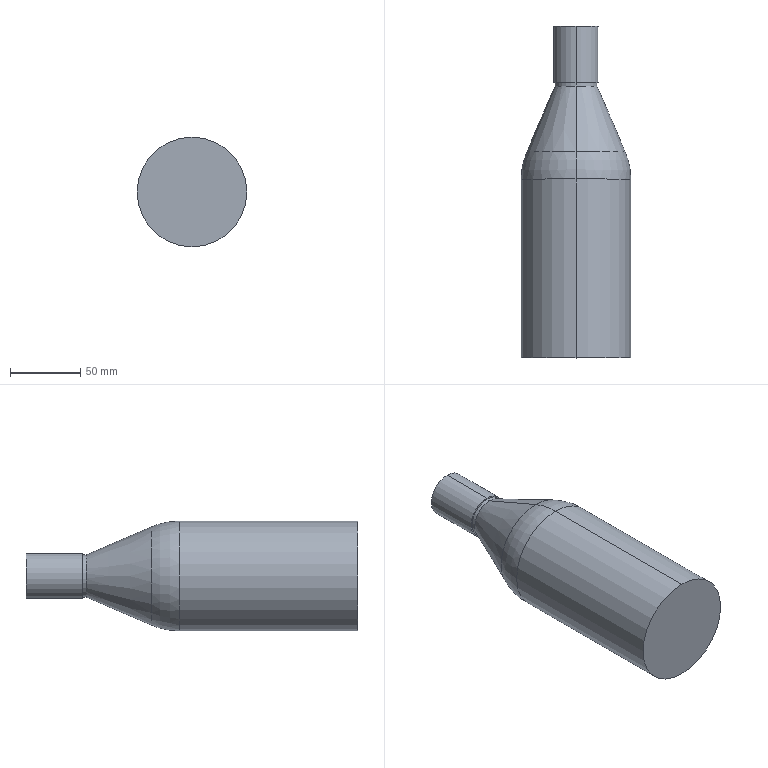Part | SolidWorks | features ICE 2, Revolution 1 | 1 solid | 21 faces | box 78 x 236 x 78 mm | volume 361829 mm3 | cylinder 10 | plane 5 | cone 4 | torus 2 | commonest cylinder face diameters 14 x2 30 x2 32 x2 62 x2 78 x2
STEP:
#1=CARTESIAN_POINT('',(0.,236.,16.));
#2=VERTEX_POINT('',#1);
#3=CARTESIAN_POINT('',(0.,236.,-16.));
#4=VERTEX_POINT('',#3);
#5=CARTESIAN_POINT('',(0.,236.,0.));
#6=DIRECTION('',(0.,1.,0.));
#7=DIRECTION('',(0.,0.,1.));
#8=AXIS2_PLACEMENT_3D('',#5,#6,#7);
#9=CIRCLE('',#8,16.);
#10=EDGE_CURVE('',#2,#4,#9,.T.);
#11=ORIENTED_EDGE('',*,*,#10,.F.);
#12=CARTESIAN_POINT('',(0.,196.,16.));
#13=VERTEX_POINT('',#12);
#14=CARTESIAN_POINT('',(0.,281.255,16.));
#15=DIRECTION('',(0.,-1.,0.));
#16=VECTOR('',#15,1000.);
#17=LINE('',#14,#16);
#18=EDGE_CURVE('',#2,#13,#17,.T.);
#19=ORIENTED_EDGE('',*,*,#18,.T.);
#20=CARTESIAN_POINT('',(0.,196.,-16.));
#21=VERTEX_POINT('',#20);
#22=CARTESIAN_POINT('',(0.,196.,0.));
#23=DIRECTION('',(0.,1.,0.));
#24=DIRECTION('',(0.,0.,1.));
#25=AXIS2_PLACEMENT_3D('',#22,#23,#24);
#26=CIRCLE('',#25,16.);
#27=EDGE_CURVE('',#13,#21,#26,.T.);
#28=ORIENTED_EDGE('',*,*,#27,.T.);
#29=CARTESIAN_POINT('',(0.,281.255,-16.));
#30=DIRECTION('',(0.,-1.,0.));
#31=VECTOR('',#30,1000.);
#32=LINE('',#29,#31);
#33=EDGE_CURVE('',#4,#21,#32,.T.);
#34=ORIENTED_EDGE('',*,*,#33,.F.);
#35=EDGE_LOOP('',(#11,#19,#28,#34));
#36=FACE_OUTER_BOUND('',#35,.T.);
#37=CARTESIAN_POINT('',(0.,281.255,0.));
#38=DIRECTION('',(0.,-1.,0.));
#39=DIRECTION('',(0.,0.,-1.));
#40=AXIS2_PLACEMENT_3D('',#37,#38,#39);
#41=CYLINDRICAL_SURFACE('',#40,16.);
#42=ADVANCED_FACE('',(#36),#41,.T.);
#43=CARTESIAN_POINT('',(0.,193.291,-15.));
#44=VERTEX_POINT('',#43);
#45=CARTESIAN_POINT('',(0.,193.291,15.));
#46=VERTEX_POINT('',#45);
#47=CARTESIAN_POINT('',(0.,193.291,0.));
#48=DIRECTION('',(0.,-1.,0.));
#49=DIRECTION('',(0.,0.,-1.));
#50=AXIS2_PLACEMENT_3D('',#47,#48,#49);
#51=CIRCLE('',#50,15.);
#52=EDGE_CURVE('',#44,#46,#51,.T.);
#53=ORIENTED_EDGE('',*,*,#52,.T.);
#54=CARTESIAN_POINT('',(0.,146.915,34.936));
#55=VERTEX_POINT('',#54);
#56=CARTESIAN_POINT('',(0.,146.915,34.936));
#57=DIRECTION('',(0.,-0.9187,0.3949));
#58=VECTOR('',#57,1000.);
#59=LINE('',#56,#58);
#60=EDGE_CURVE('',#46,#55,#59,.T.);
#61=ORIENTED_EDGE('',*,*,#60,.T.);
#62=CARTESIAN_POINT('',(0.,146.915,-34.936));
#63=VERTEX_POINT('',#62);
#64=CARTESIAN_POINT('',(0.,146.915,0.));
#65=DIRECTION('',(0.,-1.,0.));
#66=DIRECTION('',(0.,0.,-1.));
#67=AXIS2_PLACEMENT_3D('',#64,#65,#66);
#68=CIRCLE('',#67,34.936);
#69=EDGE_CURVE('',#63,#55,#68,.T.);
#70=ORIENTED_EDGE('',*,*,#69,.F.);
#71=CARTESIAN_POINT('',(0.,146.915,-34.936));
#72=DIRECTION('',(0.,-0.9187,-0.3949));
#73=VECTOR('',#72,1000.);
#74=LINE('',#71,#73);
#75=EDGE_CURVE('',#44,#63,#74,.T.);
#76=ORIENTED_EDGE('',*,*,#75,.F.);
#77=EDGE_LOOP('',(#53,#61,#70,#76));
#78=FACE_OUTER_BOUND('',#77,.T.);
#79=CARTESIAN_POINT('',(0.,146.915,0.));
#80=DIRECTION('',(0.,-1.,0.));
#81=DIRECTION('',(0.,0.,-1.));
#82=AXIS2_PLACEMENT_3D('',#79,#80,#81);
#83=CONICAL_SURFACE('',#82,34.936,0.406);
#84=ADVANCED_FACE('',(#78),#83,.T.);
#85=ORIENTED_EDGE('',*,*,#69,.T.);
#86=CARTESIAN_POINT('',(0.,127.169,39.));
#87=VERTEX_POINT('',#86);
#88=CARTESIAN_POINT('',(0.,127.169,-11.));
#89=DIRECTION('',(1.,0.,0.));
#90=DIRECTION('',(0.,0.,-1.));
#91=AXIS2_PLACEMENT_3D('',#88,#89,#90);
#92=CIRCLE('',#91,50.);
#93=EDGE_CURVE('',#55,#87,#92,.T.);
#94=ORIENTED_EDGE('',*,*,#93,.T.);
#95=CARTESIAN_POINT('',(0.,127.169,-39.));
#96=VERTEX_POINT('',#95);
#97=CARTESIAN_POINT('',(0.,127.169,0.));
#98=DIRECTION('',(0.,-1.,0.));
#99=DIRECTION('',(0.,0.,-1.));
#100=AXIS2_PLACEMENT_3D('',#97,#98,#99);
#101=CIRCLE('',#100,39.);
#102=EDGE_CURVE('',#96,#87,#101,.T.);
#103=ORIENTED_EDGE('',*,*,#102,.F.);
#104=CARTESIAN_POINT('',(0.,127.169,11.));
#105=DIRECTION('',(-1.,0.,0.));
#106=DIRECTION('',(0.,0.,1.));
#107=AXIS2_PLACEMENT_3D('',#104,#105,#106);
#108=CIRCLE('',#107,50.);
#109=EDGE_CURVE('',#63,#96,#108,.T.);
#110=ORIENTED_EDGE('',*,*,#109,.F.);
#111=EDGE_LOOP('',(#85,#94,#103,#110));
#112=FACE_OUTER_BOUND('',#111,.T.);
#113=CARTESIAN_POINT('',(0.,127.169,0.));
#114=DIRECTION('',(0.,-1.,0.));
#115=DIRECTION('',(0.,0.,-1.));
#116=AXIS2_PLACEMENT_3D('',#113,#114,#115);
#117=TOROIDAL_SURFACE('',#116,-11.,50.);
#118=ADVANCED_FACE('',(#112),#117,.T.);
#119=ORIENTED_EDGE('',*,*,#102,.T.);
#120=CARTESIAN_POINT('',(0.,0.,39.));
#121=VERTEX_POINT('',#120);
#122=CARTESIAN_POINT('',(0.,0.,39.));
#123=DIRECTION('',(0.,-1.,0.));
#124=VECTOR('',#123,1000.);
#125=LINE('',#122,#124);
#126=EDGE_CURVE('',#87,#121,#125,.T.);
#127=ORIENTED_EDGE('',*,*,#126,.T.);
#128=CARTESIAN_POINT('',(0.,0.,-39.));
#129=VERTEX_POINT('',#128);
#130=CARTESIAN_POINT('',(0.,0.,0.));
#131=DIRECTION('',(0.,-1.,0.));
#132=DIRECTION('',(0.,0.,-1.));
#133=AXIS2_PLACEMENT_3D('',#130,#131,#132);
#134=CIRCLE('',#133,39.);
#135=EDGE_CURVE('',#129,#121,#134,.T.);
#136=ORIENTED_EDGE('',*,*,#135,.F.);
#137=CARTESIAN_POINT('',(0.,0.,-39.));
#138=DIRECTION('',(0.,-1.,0.));
#139=VECTOR('',#138,1000.);
#140=LINE('',#137,#139);
#141=EDGE_CURVE('',#96,#129,#140,.T.);
#142=ORIENTED_EDGE('',*,*,#141,.F.);
#143=EDGE_LOOP('',(#119,#127,#136,#142));
#144=FACE_OUTER_BOUND('',#143,.T.);
#145=CARTESIAN_POINT('',(0.,0.,0.));
#146=DIRECTION('',(0.,-1.,0.));
#147=DIRECTION('',(0.,0.,-1.));
#148=AXIS2_PLACEMENT_3D('',#145,#146,#147);
#149=CYLINDRICAL_SURFACE('',#148,39.);
#150=ADVANCED_FACE('',(#144),#149,.T.);
#151=CARTESIAN_POINT('',(0.,196.,15.));
#152=VERTEX_POINT('',#151);
#153=CARTESIAN_POINT('',(0.,196.,-15.));
#154=VERTEX_POINT('',#153);
#155=CARTESIAN_POINT('',(0.,196.,0.));
#156=DIRECTION('',(0.,1.,0.));
#157=DIRECTION('',(0.,0.,1.));
#158=AXIS2_PLACEMENT_3D('',#155,#156,#157);
#159=CIRCLE('',#158,15.);
#160=EDGE_CURVE('',#152,#154,#159,.T.);
#161=ORIENTED_EDGE('',*,*,#160,.F.);
#162=CARTESIAN_POINT('',(0.,0.,15.));
#163=DIRECTION('',(0.,-1.,0.));
#164=VECTOR('',#163,1000.);
#165=LINE('',#162,#164);
#166=EDGE_CURVE('',#152,#46,#165,.T.);
#167=ORIENTED_EDGE('',*,*,#166,.T.);
#168=ORIENTED_EDGE('',*,*,#52,.F.);
#169=CARTESIAN_POINT('',(0.,0.,-15.));
#170=DIRECTION('',(0.,-1.,0.));
#171=VECTOR('',#170,1000.);
#172=LINE('',#169,#171);
#173=EDGE_CURVE('',#154,#44,#172,.T.);
#174=ORIENTED_EDGE('',*,*,#173,.F.);
#175=EDGE_LOOP('',(#161,#167,#168,#174));
#176=FACE_OUTER_BOUND('',#175,.T.);
#177=CARTESIAN_POINT('',(0.,0.,0.));
#178=DIRECTION('',(0.,-1.,0.));
#179=DIRECTION('',(0.,0.,-1.));
#180=AXIS2_PLACEMENT_3D('',#177,#178,#179);
#181=CYLINDRICAL_SURFACE('',#180,15.);
#182=ADVANCED_FACE('',(#176),#181,.T.);
#183=ORIENTED_EDGE('',*,*,#166,.F.);
#184=CARTESIAN_POINT('',(0.,196.,0.));
#185=DIRECTION('',(0.,1.,0.));
#186=DIRECTION('',(0.,0.,1.));
#187=AXIS2_PLACEMENT_3D('',#184,#185,#186);
#188=CIRCLE('',#187,15.);
#189=EDGE_CURVE('',#154,#152,#188,.T.);
#190=ORIENTED_EDGE('',*,*,#189,.F.);
#191=ORIENTED_EDGE('',*,*,#173,.T.);
#192=CARTESIAN_POINT('',(0.,193.291,0.));
#193=DIRECTION('',(0.,-1.,0.));
#194=DIRECTION('',(0.,0.,-1.));
#195=AXIS2_PLACEMENT_3D('',#192,#193,#194);
#196=CIRCLE('',#195,15.);
#197=EDGE_CURVE('',#46,#44,#196,.T.);
#198=ORIENTED_EDGE('',*,*,#197,.F.);
#199=EDGE_LOOP('',(#183,#190,#191,#198));
#200=FACE_OUTER_BOUND('',#199,.T.);
#201=CARTESIAN_POINT('',(0.,0.,0.));
#202=DIRECTION('',(0.,-1.,0.));
#203=DIRECTION('',(0.,0.,-1.));
#204=AXIS2_PLACEMENT_3D('',#201,#202,#203);
#205=CYLINDRICAL_SURFACE('',#204,15.);
#206=ADVANCED_FACE('',(#200),#205,.T.);
#207=ORIENTED_EDGE('',*,*,#135,.T.);
#208=CARTESIAN_POINT('',(0.,0.,0.));
#209=DIRECTION('',(0.,-1.,0.));
#210=DIRECTION('',(0.,0.,-1.));
#211=AXIS2_PLACEMENT_3D('',#208,#209,#210);
#212=CIRCLE('',#211,39.);
#213=EDGE_CURVE('',#121,#129,#212,.T.);
#214=ORIENTED_EDGE('',*,*,#213,.T.);
#215=EDGE_LOOP('',(#207,#214));
#216=FACE_OUTER_BOUND('',#215,.T.);
#217=CARTESIAN_POINT('',(0.,0.,0.));
#218=DIRECTION('',(0.,-1.,0.));
#219=DIRECTION('',(0.,0.,-1.));
#220=AXIS2_PLACEMENT_3D('',#217,#218,#219);
#221=PLANE('',#220);
#222=ADVANCED_FACE('',(#216),#221,.T.);
#223=ORIENTED_EDGE('',*,*,#126,.F.);
#224=CARTESIAN_POINT('',(0.,127.169,0.));
#225=DIRECTION('',(0.,-1.,0.));
#226=DIRECTION('',(0.,0.,-1.));
#227=AXIS2_PLACEMENT_3D('',#224,#225,#226);
#228=CIRCLE('',#227,39.);
#229=EDGE_CURVE('',#87,#96,#228,.T.);
#230=ORIENTED_EDGE('',*,*,#229,.T.);
#231=ORIENTED_EDGE('',*,*,#141,.T.);
#232=ORIENTED_EDGE('',*,*,#213,.F.);
#233=EDGE_LOOP('',(#223,#230,#231,#232));
#234=FACE_OUTER_BOUND('',#233,.T.);
#235=CARTESIAN_POINT('',(0.,0.,0.));
#236=DIRECTION('',(0.,-1.,0.));
#237=DIRECTION('',(0.,0.,-1.));
#238=AXIS2_PLACEMENT_3D('',#235,#236,#237);
#239=CYLINDRICAL_SURFACE('',#238,39.);
#240=ADVANCED_FACE('',(#234),#239,.T.);
#241=ORIENTED_EDGE('',*,*,#93,.F.);
#242=CARTESIAN_POINT('',(0.,146.915,0.));
#243=DIRECTION('',(0.,-1.,0.));
#244=DIRECTION('',(0.,0.,-1.));
#245=AXIS2_PLACEMENT_3D('',#242,#243,#244);
#246=CIRCLE('',#245,34.936);
#247=EDGE_CURVE('',#55,#63,#246,.T.);
#248=ORIENTED_EDGE('',*,*,#247,.T.);
#249=ORIENTED_EDGE('',*,*,#109,.T.);
#250=ORIENTED_EDGE('',*,*,#229,.F.);
#251=EDGE_LOOP('',(#241,#248,#249,#250));
#252=FACE_OUTER_BOUND('',#251,.T.);
#253=CARTESIAN_POINT('',(0.,127.169,0.));
#254=DIRECTION('',(0.,-1.,0.));
#255=DIRECTION('',(0.,0.,-1.));
#256=AXIS2_PLACEMENT_3D('',#253,#254,#255);
#257=TOROIDAL_SURFACE('',#256,-11.,50.);
#258=ADVANCED_FACE('',(#252),#257,.T.);
#259=ORIENTED_EDGE('',*,*,#60,.F.);
#260=ORIENTED_EDGE('',*,*,#197,.T.);
#261=ORIENTED_EDGE('',*,*,#75,.T.);
#262=ORIENTED_EDGE('',*,*,#247,.F.);
#263=EDGE_LOOP('',(#259,#260,#261,#262));
#264=FACE_OUTER_BOUND('',#263,.T.);
#265=CARTESIAN_POINT('',(0.,146.915,0.));
#266=DIRECTION('',(0.,-1.,0.));
#267=DIRECTION('',(0.,0.,-1.));
#268=AXIS2_PLACEMENT_3D('',#265,#266,#267);
#269=CONICAL_SURFACE('',#268,34.936,0.406);
#270=ADVANCED_FACE('',(#264),#269,.T.);
#271=ORIENTED_EDGE('',*,*,#18,.F.);
#272=CARTESIAN_POINT('',(0.,236.,0.));
#273=DIRECTION('',(0.,1.,0.));
#274=DIRECTION('',(0.,0.,1.));
#275=AXIS2_PLACEMENT_3D('',#272,#273,#274);
#276=CIRCLE('',#275,16.);
#277=EDGE_CURVE('',#4,#2,#276,.T.);
#278=ORIENTED_EDGE('',*,*,#277,.F.);
#279=ORIENTED_EDGE('',*,*,#33,.T.);
#280=CARTESIAN_POINT('',(0.,196.,0.));
#281=DIRECTION('',(0.,1.,0.));
#282=DIRECTION('',(0.,0.,1.));
#283=AXIS2_PLACEMENT_3D('',#280,#281,#282);
#284=CIRCLE('',#283,16.);
#285=EDGE_CURVE('',#21,#13,#284,.T.);
#286=ORIENTED_EDGE('',*,*,#285,.T.);
#287=EDGE_LOOP('',(#271,#278,#279,#286));
#288=FACE_OUTER_BOUND('',#287,.T.);
#289=CARTESIAN_POINT('',(0.,281.255,0.));
#290=DIRECTION('',(0.,-1.,0.));
#291=DIRECTION('',(0.,0.,-1.));
#292=AXIS2_PLACEMENT_3D('',#289,#290,#291);
#293=CYLINDRICAL_SURFACE('',#292,16.);
#294=ADVANCED_FACE('',(#288),#293,.T.);
#295=ORIENTED_EDGE('',*,*,#285,.F.);
#296=ORIENTED_EDGE('',*,*,#27,.F.);
#297=EDGE_LOOP('',(#295,#296));
#298=FACE_OUTER_BOUND('',#297,.T.);
#299=ORIENTED_EDGE('',*,*,#189,.T.);
#300=ORIENTED_EDGE('',*,*,#160,.T.);
#301=EDGE_LOOP('',(#299,#300));
#302=FACE_BOUND('',#301,.T.);
#303=CARTESIAN_POINT('',(0.,196.,0.));
#304=DIRECTION('',(0.,1.,0.));
#305=DIRECTION('',(0.,0.,1.));
#306=AXIS2_PLACEMENT_3D('',#303,#304,#305);
#307=PLANE('',#306);
#308=ADVANCED_FACE('',(#298,#302),#307,.F.);
#309=ORIENTED_EDGE('',*,*,#277,.T.);
#310=ORIENTED_EDGE('',*,*,#10,.T.);
#311=EDGE_LOOP('',(#309,#310));
#312=FACE_OUTER_BOUND('',#311,.T.);
#313=CARTESIAN_POINT('',(7.,236.,0.));
#314=DIRECTION('',(0.,1.,0.));
#315=DIRECTION('',(0.,0.,1.));
#316=AXIS2_PLACEMENT_3D('',#313,#314,#315);
#317=PLANE('',#316);
#318=ADVANCED_FACE('',(#312),#317,.T.);
#319=CLOSED_SHELL('',(#42,#84,#118,#150,#182,#206,#222,#240,#258,#270,#294,#308,#318));
#320=CARTESIAN_POINT('',(0.,231.,-7.));
#321=VERTEX_POINT('',#320);
#322=CARTESIAN_POINT('',(0.,231.,7.));
#323=VERTEX_POINT('',#322);
#324=CARTESIAN_POINT('',(0.,231.,0.));
#325=DIRECTION('',(0.,1.,0.));
#326=DIRECTION('',(0.,0.,1.));
#327=AXIS2_PLACEMENT_3D('',#324,#325,#326);
#328=CIRCLE('',#327,7.);
#329=EDGE_CURVE('',#321,#323,#328,.T.);
#330=ORIENTED_EDGE('',*,*,#329,.T.);
#331=CARTESIAN_POINT('',(0.,191.644,7.));
#332=VERTEX_POINT('',#331);
#333=CARTESIAN_POINT('',(0.,0.,7.));
#334=DIRECTION('',(0.,-1.,0.));
#335=VECTOR('',#334,1000.);
#336=LINE('',#333,#335);
#337=EDGE_CURVE('',#323,#332,#336,.T.);
#338=ORIENTED_EDGE('',*,*,#337,.T.);
#339=CARTESIAN_POINT('',(0.,191.644,-7.));
#340=VERTEX_POINT('',#339);
#341=CARTESIAN_POINT('',(0.,191.644,0.));
#342=DIRECTION('',(0.,-1.,0.));
#343=DIRECTION('',(0.,0.,-1.));
#344=AXIS2_PLACEMENT_3D('',#341,#342,#343);
#345=CIRCLE('',#344,7.);
#346=EDGE_CURVE('',#332,#340,#345,.T.);
#347=ORIENTED_EDGE('',*,*,#346,.T.);
#348=CARTESIAN_POINT('',(0.,0.,-7.));
#349=DIRECTION('',(0.,-1.,0.));
#350=VECTOR('',#349,1000.);
#351=LINE('',#348,#350);
#352=EDGE_CURVE('',#321,#340,#351,.T.);
#353=ORIENTED_EDGE('',*,*,#352,.F.);
#354=EDGE_LOOP('',(#330,#338,#347,#353));
#355=FACE_OUTER_BOUND('',#354,.T.);
#356=CARTESIAN_POINT('',(0.,0.,0.));
#357=DIRECTION('',(0.,-1.,0.));
#358=DIRECTION('',(0.,0.,-1.));
#359=AXIS2_PLACEMENT_3D('',#356,#357,#358);
#360=CYLINDRICAL_SURFACE('',#359,7.);
#361=ADVANCED_FACE('',(#355),#360,.F.);
#362=ORIENTED_EDGE('',*,*,#346,.F.);
#363=CARTESIAN_POINT('',(0.,135.813,31.));
#364=VERTEX_POINT('',#363);
#365=CARTESIAN_POINT('',(0.,191.644,7.));
#366=DIRECTION('',(0.,-0.9187,0.3949));
#367=VECTOR('',#366,1000.);
#368=LINE('',#365,#367);
#369=EDGE_CURVE('',#332,#364,#368,.T.);
#370=ORIENTED_EDGE('',*,*,#369,.T.);
#371=CARTESIAN_POINT('',(0.,135.813,-31.));
#372=VERTEX_POINT('',#371);
#373=CARTESIAN_POINT('',(0.,135.813,0.));
#374=DIRECTION('',(0.,-1.,0.));
#375=DIRECTION('',(0.,0.,-1.));
#376=AXIS2_PLACEMENT_3D('',#373,#374,#375);
#377=CIRCLE('',#376,31.);
#378=EDGE_CURVE('',#364,#372,#377,.T.);
#379=ORIENTED_EDGE('',*,*,#378,.T.);
#380=CARTESIAN_POINT('',(0.,191.644,-7.));
#381=DIRECTION('',(0.,-0.9187,-0.3949));
#382=VECTOR('',#381,1000.);
#383=LINE('',#380,#382);
#384=EDGE_CURVE('',#340,#372,#383,.T.);
#385=ORIENTED_EDGE('',*,*,#384,.F.);
#386=EDGE_LOOP('',(#362,#370,#379,#385));
#387=FACE_OUTER_BOUND('',#386,.T.);
#388=CARTESIAN_POINT('',(0.,191.644,0.));
#389=DIRECTION('',(0.,-1.,0.));
#390=DIRECTION('',(0.,0.,-1.));
#391=AXIS2_PLACEMENT_3D('',#388,#389,#390);
#392=CONICAL_SURFACE('',#391,7.,0.406);
#393=ADVANCED_FACE('',(#387),#392,.F.);
#394=ORIENTED_EDGE('',*,*,#378,.F.);
#395=CARTESIAN_POINT('',(0.,8.,31.));
#396=VERTEX_POINT('',#395);
#397=CARTESIAN_POINT('',(0.,0.,31.));
#398=DIRECTION('',(0.,-1.,0.));
#399=VECTOR('',#398,1000.);
#400=LINE('',#397,#399);
#401=EDGE_CURVE('',#364,#396,#400,.T.);
#402=ORIENTED_EDGE('',*,*,#401,.T.);
#403=CARTESIAN_POINT('',(0.,8.,-31.));
#404=VERTEX_POINT('',#403);
#405=CARTESIAN_POINT('',(0.,8.,0.));
#406=DIRECTION('',(0.,-1.,0.));
#407=DIRECTION('',(0.,0.,-1.));
#408=AXIS2_PLACEMENT_3D('',#405,#406,#407);
#409=CIRCLE('',#408,31.);
#410=EDGE_CURVE('',#396,#404,#409,.T.);
#411=ORIENTED_EDGE('',*,*,#410,.T.);
#412=CARTESIAN_POINT('',(0.,0.,-31.));
#413=DIRECTION('',(0.,-1.,0.));
#414=VECTOR('',#413,1000.);
#415=LINE('',#412,#414);
#416=EDGE_CURVE('',#372,#404,#415,.T.);
#417=ORIENTED_EDGE('',*,*,#416,.F.);
#418=EDGE_LOOP('',(#394,#402,#411,#417));
#419=FACE_OUTER_BOUND('',#418,.T.);
#420=CARTESIAN_POINT('',(0.,0.,0.));
#421=DIRECTION('',(0.,-1.,0.));
#422=DIRECTION('',(0.,0.,-1.));
#423=AXIS2_PLACEMENT_3D('',#420,#421,#422);
#424=CYLINDRICAL_SURFACE('',#423,31.);
#425=ADVANCED_FACE('',(#419),#424,.F.);
#426=ORIENTED_EDGE('',*,*,#329,.F.);
#427=CARTESIAN_POINT('',(0.,231.,0.));
#428=DIRECTION('',(0.,1.,0.));
#429=DIRECTION('',(0.,0.,1.));
#430=AXIS2_PLACEMENT_3D('',#427,#428,#429);
#431=CIRCLE('',#430,7.);
#432=EDGE_CURVE('',#323,#321,#431,.T.);
#433=ORIENTED_EDGE('',*,*,#432,.F.);
#434=EDGE_LOOP('',(#426,#433));
#435=FACE_OUTER_BOUND('',#434,.T.);
#436=CARTESIAN_POINT('',(0.,231.,0.));
#437=DIRECTION('',(0.,1.,0.));
#438=DIRECTION('',(0.,0.,1.));
#439=AXIS2_PLACEMENT_3D('',#436,#437,#438);
#440=PLANE('',#439);
#441=ADVANCED_FACE('',(#435),#440,.F.);
#442=CARTESIAN_POINT('',(0.,8.,0.));
#443=DIRECTION('',(0.,-1.,0.));
#444=DIRECTION('',(0.,0.,-1.));
#445=AXIS2_PLACEMENT_3D('',#442,#443,#444);
#446=CIRCLE('',#445,31.);
#447=EDGE_CURVE('',#404,#396,#446,.T.);
#448=ORIENTED_EDGE('',*,*,#447,.F.);
#449=ORIENTED_EDGE('',*,*,#410,.F.);
#450=EDGE_LOOP('',(#448,#449));
#451=FACE_OUTER_BOUND('',#450,.T.);
#452=CARTESIAN_POINT('',(0.,8.,0.));
#453=DIRECTION('',(0.,1.,0.));
#454=DIRECTION('',(0.,0.,1.));
#455=AXIS2_PLACEMENT_3D('',#452,#453,#454);
#456=PLANE('',#455);
#457=ADVANCED_FACE('',(#451),#456,.T.);
#458=ORIENTED_EDGE('',*,*,#401,.F.);
#459=CARTESIAN_POINT('',(0.,135.813,0.));
#460=DIRECTION('',(0.,-1.,0.));
#461=DIRECTION('',(0.,0.,-1.));
#462=AXIS2_PLACEMENT_3D('',#459,#460,#461);
#463=CIRCLE('',#462,31.);
#464=EDGE_CURVE('',#372,#364,#463,.T.);
#465=ORIENTED_EDGE('',*,*,#464,.F.);
#466=ORIENTED_EDGE('',*,*,#416,.T.);
#467=ORIENTED_EDGE('',*,*,#447,.T.);
#468=EDGE_LOOP('',(#458,#465,#466,#467));
#469=FACE_OUTER_BOUND('',#468,.T.);
#470=CARTESIAN_POINT('',(0.,0.,0.));
#471=DIRECTION('',(0.,-1.,0.));
#472=DIRECTION('',(0.,0.,-1.));
#473=AXIS2_PLACEMENT_3D('',#470,#471,#472);
#474=CYLINDRICAL_SURFACE('',#473,31.);
#475=ADVANCED_FACE('',(#469),#474,.F.);
#476=ORIENTED_EDGE('',*,*,#369,.F.);
#477=CARTESIAN_POINT('',(0.,191.644,0.));
#478=DIRECTION('',(0.,-1.,0.));
#479=DIRECTION('',(0.,0.,-1.));
#480=AXIS2_PLACEMENT_3D('',#477,#478,#479);
#481=CIRCLE('',#480,7.);
#482=EDGE_CURVE('',#340,#332,#481,.T.);
#483=ORIENTED_EDGE('',*,*,#482,.F.);
#484=ORIENTED_EDGE('',*,*,#384,.T.);
#485=ORIENTED_EDGE('',*,*,#464,.T.);
#486=EDGE_LOOP('',(#476,#483,#484,#485));
#487=FACE_OUTER_BOUND('',#486,.T.);
#488=CARTESIAN_POINT('',(0.,191.644,0.));
#489=DIRECTION('',(0.,-1.,0.));
#490=DIRECTION('',(0.,0.,-1.));
#491=AXIS2_PLACEMENT_3D('',#488,#489,#490);
#492=CONICAL_SURFACE('',#491,7.,0.406);
#493=ADVANCED_FACE('',(#487),#492,.F.);
#494=ORIENTED_EDGE('',*,*,#337,.F.);
#495=ORIENTED_EDGE('',*,*,#432,.T.);
#496=ORIENTED_EDGE('',*,*,#352,.T.);
#497=ORIENTED_EDGE('',*,*,#482,.T.);
#498=EDGE_LOOP('',(#494,#495,#496,#497));
#499=FACE_OUTER_BOUND('',#498,.T.);
#500=CARTESIAN_POINT('',(0.,0.,0.));
#501=DIRECTION('',(0.,-1.,0.));
#502=DIRECTION('',(0.,0.,-1.));
#503=AXIS2_PLACEMENT_3D('',#500,#501,#502);
#504=CYLINDRICAL_SURFACE('',#503,7.);
#505=ADVANCED_FACE('',(#499),#504,.F.);
#506=CLOSED_SHELL('',(#361,#393,#425,#441,#457,#475,#493,#505));
#507=ORIENTED_CLOSED_SHELL('',*,#506,.F.);
#508=BREP_WITH_VOIDS('',#319,(#507));
#509=CARTESIAN_POINT('',(0.,0.,0.));
#510=DIRECTION('',(0.,0.,1.));
#511=DIRECTION('',(1.,0.,0.));
#512=AXIS2_PLACEMENT_3D('',#509,#510,#511);
#513=(LENGTH_UNIT()NAMED_UNIT(*)SI_UNIT(.MILLI.,.METRE.));
#514=UNCERTAINTY_MEASURE_WITH_UNIT(LENGTH_MEASURE(0.00001),#513,'','');
#515=(NAMED_UNIT(*)PLANE_ANGLE_UNIT()SI_UNIT($,.RADIAN.));
#516=(NAMED_UNIT(*)SI_UNIT($,.STERADIAN.)SOLID_ANGLE_UNIT());
#517=(GEOMETRIC_REPRESENTATION_CONTEXT(3)GLOBAL_UNCERTAINTY_ASSIGNED_CONTEXT((#514))GLOBAL_UNIT_ASSIGNED_CONTEXT((#513,#515,#516))REPRESENTATION_CONTEXT('',''));
#518=ADVANCED_BREP_SHAPE_REPRESENTATION('',(#508,#512),#517);